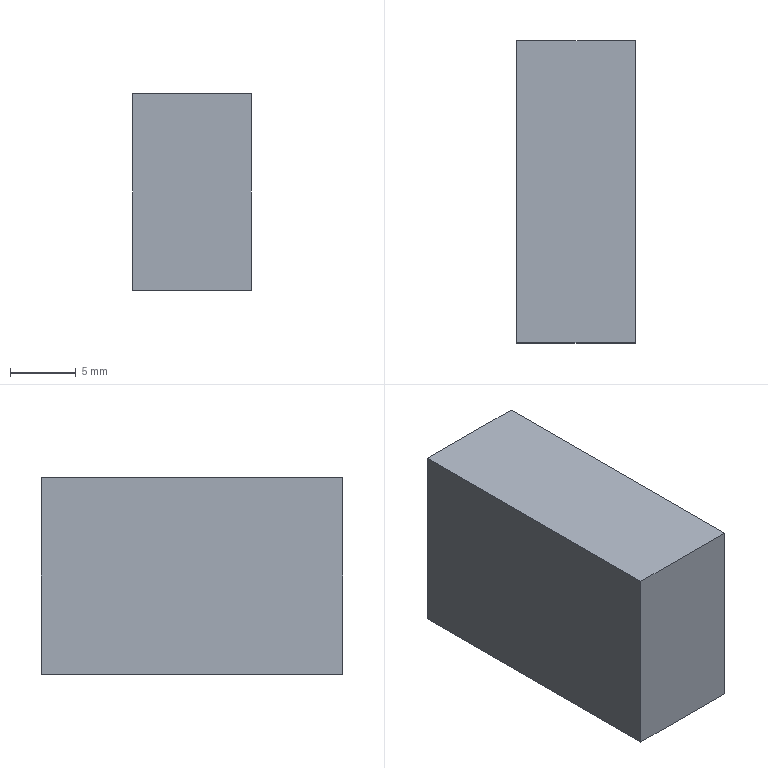Part | STEP file | 11-sy5120-5gz-01_sy51802operend-V2.0-V2.011_SingleB | 1 solid | 6 faces | box 9 x 23 x 15 mm | volume 3105 mm3 | plane 6
STEP:
#1=CARTESIAN_POINT('',(-9.,0.,7.5));
#2=VERTEX_POINT('',#1);
#3=CARTESIAN_POINT('',(-9.,0.,-7.5));
#4=VERTEX_POINT('',#3);
#5=CARTESIAN_POINT('',(-9.,0.,7.5));
#6=DIRECTION('',(0.,0.,-1.));
#7=VECTOR('',#6,1000.);
#8=LINE('',#5,#7);
#9=EDGE_CURVE('',#2,#4,#8,.T.);
#10=ORIENTED_EDGE('',*,*,#9,.T.);
#11=CARTESIAN_POINT('',(0.,0.,-7.5));
#12=VERTEX_POINT('',#11);
#13=CARTESIAN_POINT('',(-9.,0.,-7.5));
#14=DIRECTION('',(1.,0.,0.));
#15=VECTOR('',#14,1000.);
#16=LINE('',#13,#15);
#17=EDGE_CURVE('',#4,#12,#16,.T.);
#18=ORIENTED_EDGE('',*,*,#17,.T.);
#19=CARTESIAN_POINT('',(0.,0.,7.5));
#20=VERTEX_POINT('',#19);
#21=CARTESIAN_POINT('',(0.,0.,7.5));
#22=DIRECTION('',(0.,0.,-1.));
#23=VECTOR('',#22,1000.);
#24=LINE('',#21,#23);
#25=EDGE_CURVE('',#20,#12,#24,.T.);
#26=ORIENTED_EDGE('',*,*,#25,.F.);
#27=CARTESIAN_POINT('',(-9.,0.,7.5));
#28=DIRECTION('',(1.,0.,0.));
#29=VECTOR('',#28,1000.);
#30=LINE('',#27,#29);
#31=EDGE_CURVE('',#2,#20,#30,.T.);
#32=ORIENTED_EDGE('',*,*,#31,.F.);
#33=EDGE_LOOP('',(#10,#18,#26,#32));
#34=FACE_OUTER_BOUND('',#33,.T.);
#35=CARTESIAN_POINT('',(-9.,0.,7.5));
#36=DIRECTION('',(0.,1.,0.));
#37=DIRECTION('',(0.,0.,1.));
#38=AXIS2_PLACEMENT_3D('',#35,#36,#37);
#39=PLANE('',#38);
#40=ADVANCED_FACE('',(#34),#39,.F.);
#41=ORIENTED_EDGE('',*,*,#25,.T.);
#42=CARTESIAN_POINT('',(0.,23.,-7.5));
#43=VERTEX_POINT('',#42);
#44=CARTESIAN_POINT('',(0.,0.,-7.5));
#45=DIRECTION('',(0.,1.,0.));
#46=VECTOR('',#45,1000.);
#47=LINE('',#44,#46);
#48=EDGE_CURVE('',#12,#43,#47,.T.);
#49=ORIENTED_EDGE('',*,*,#48,.T.);
#50=CARTESIAN_POINT('',(0.,23.,7.5));
#51=VERTEX_POINT('',#50);
#52=CARTESIAN_POINT('',(0.,23.,7.5));
#53=DIRECTION('',(0.,0.,-1.));
#54=VECTOR('',#53,1000.);
#55=LINE('',#52,#54);
#56=EDGE_CURVE('',#51,#43,#55,.T.);
#57=ORIENTED_EDGE('',*,*,#56,.F.);
#58=CARTESIAN_POINT('',(0.,0.,7.5));
#59=DIRECTION('',(0.,1.,0.));
#60=VECTOR('',#59,1000.);
#61=LINE('',#58,#60);
#62=EDGE_CURVE('',#20,#51,#61,.T.);
#63=ORIENTED_EDGE('',*,*,#62,.F.);
#64=EDGE_LOOP('',(#41,#49,#57,#63));
#65=FACE_OUTER_BOUND('',#64,.T.);
#66=CARTESIAN_POINT('',(0.,0.,7.5));
#67=DIRECTION('',(-1.,0.,0.));
#68=DIRECTION('',(0.,-1.,0.));
#69=AXIS2_PLACEMENT_3D('',#66,#67,#68);
#70=PLANE('',#69);
#71=ADVANCED_FACE('',(#65),#70,.F.);
#72=ORIENTED_EDGE('',*,*,#56,.T.);
#73=CARTESIAN_POINT('',(-9.,23.,-7.5));
#74=VERTEX_POINT('',#73);
#75=CARTESIAN_POINT('',(0.,23.,-7.5));
#76=DIRECTION('',(-1.,0.,0.));
#77=VECTOR('',#76,1000.);
#78=LINE('',#75,#77);
#79=EDGE_CURVE('',#43,#74,#78,.T.);
#80=ORIENTED_EDGE('',*,*,#79,.T.);
#81=CARTESIAN_POINT('',(-9.,23.,7.5));
#82=VERTEX_POINT('',#81);
#83=CARTESIAN_POINT('',(-9.,23.,7.5));
#84=DIRECTION('',(0.,0.,-1.));
#85=VECTOR('',#84,1000.);
#86=LINE('',#83,#85);
#87=EDGE_CURVE('',#82,#74,#86,.T.);
#88=ORIENTED_EDGE('',*,*,#87,.F.);
#89=CARTESIAN_POINT('',(0.,23.,7.5));
#90=DIRECTION('',(-1.,0.,0.));
#91=VECTOR('',#90,1000.);
#92=LINE('',#89,#91);
#93=EDGE_CURVE('',#51,#82,#92,.T.);
#94=ORIENTED_EDGE('',*,*,#93,.F.);
#95=EDGE_LOOP('',(#72,#80,#88,#94));
#96=FACE_OUTER_BOUND('',#95,.T.);
#97=CARTESIAN_POINT('',(0.,23.,7.5));
#98=DIRECTION('',(0.,-1.,0.));
#99=DIRECTION('',(1.,0.,0.));
#100=AXIS2_PLACEMENT_3D('',#97,#98,#99);
#101=PLANE('',#100);
#102=ADVANCED_FACE('',(#96),#101,.F.);
#103=ORIENTED_EDGE('',*,*,#87,.T.);
#104=CARTESIAN_POINT('',(-9.,23.,-7.5));
#105=DIRECTION('',(0.,-1.,0.));
#106=VECTOR('',#105,1000.);
#107=LINE('',#104,#106);
#108=EDGE_CURVE('',#74,#4,#107,.T.);
#109=ORIENTED_EDGE('',*,*,#108,.T.);
#110=ORIENTED_EDGE('',*,*,#9,.F.);
#111=CARTESIAN_POINT('',(-9.,23.,7.5));
#112=DIRECTION('',(0.,-1.,0.));
#113=VECTOR('',#112,1000.);
#114=LINE('',#111,#113);
#115=EDGE_CURVE('',#82,#2,#114,.T.);
#116=ORIENTED_EDGE('',*,*,#115,.F.);
#117=EDGE_LOOP('',(#103,#109,#110,#116));
#118=FACE_OUTER_BOUND('',#117,.T.);
#119=CARTESIAN_POINT('',(-9.,23.,7.5));
#120=DIRECTION('',(1.,0.,0.));
#121=DIRECTION('',(0.,1.,0.));
#122=AXIS2_PLACEMENT_3D('',#119,#120,#121);
#123=PLANE('',#122);
#124=ADVANCED_FACE('',(#118),#123,.F.);
#125=ORIENTED_EDGE('',*,*,#31,.T.);
#126=ORIENTED_EDGE('',*,*,#62,.T.);
#127=ORIENTED_EDGE('',*,*,#93,.T.);
#128=ORIENTED_EDGE('',*,*,#115,.T.);
#129=EDGE_LOOP('',(#125,#126,#127,#128));
#130=FACE_OUTER_BOUND('',#129,.T.);
#131=CARTESIAN_POINT('',(-9.,0.,7.5));
#132=DIRECTION('',(0.,0.,-1.));
#133=DIRECTION('',(-1.,0.,0.));
#134=AXIS2_PLACEMENT_3D('',#131,#132,#133);
#135=PLANE('',#134);
#136=ADVANCED_FACE('',(#130),#135,.F.);
#137=ORIENTED_EDGE('',*,*,#17,.F.);
#138=ORIENTED_EDGE('',*,*,#108,.F.);
#139=ORIENTED_EDGE('',*,*,#79,.F.);
#140=ORIENTED_EDGE('',*,*,#48,.F.);
#141=EDGE_LOOP('',(#137,#138,#139,#140));
#142=FACE_OUTER_BOUND('',#141,.T.);
#143=CARTESIAN_POINT('',(-9.,0.,-7.5));
#144=DIRECTION('',(0.,0.,-1.));
#145=DIRECTION('',(-1.,0.,0.));
#146=AXIS2_PLACEMENT_3D('',#143,#144,#145);
#147=PLANE('',#146);
#148=ADVANCED_FACE('',(#142),#147,.T.);
#149=CLOSED_SHELL('',(#40,#71,#102,#124,#136,#148));
#150=MANIFOLD_SOLID_BREP('',#149);
#151=CARTESIAN_POINT('',(0.,0.,0.));
#152=DIRECTION('',(0.,0.,1.));
#153=DIRECTION('',(1.,0.,0.));
#154=AXIS2_PLACEMENT_3D('',#151,#152,#153);
#155=(LENGTH_UNIT()NAMED_UNIT(*)SI_UNIT(.MILLI.,.METRE.));
#156=UNCERTAINTY_MEASURE_WITH_UNIT(LENGTH_MEASURE(0.00001),#155,'','');
#157=(NAMED_UNIT(*)PLANE_ANGLE_UNIT()SI_UNIT($,.RADIAN.));
#158=(NAMED_UNIT(*)SI_UNIT($,.STERADIAN.)SOLID_ANGLE_UNIT());
#159=(GEOMETRIC_REPRESENTATION_CONTEXT(3)GLOBAL_UNCERTAINTY_ASSIGNED_CONTEXT((#156))GLOBAL_UNIT_ASSIGNED_CONTEXT((#155,#157,#158))REPRESENTATION_CONTEXT('',''));
#160=ADVANCED_BREP_SHAPE_REPRESENTATION('',(#150,#154),#159);